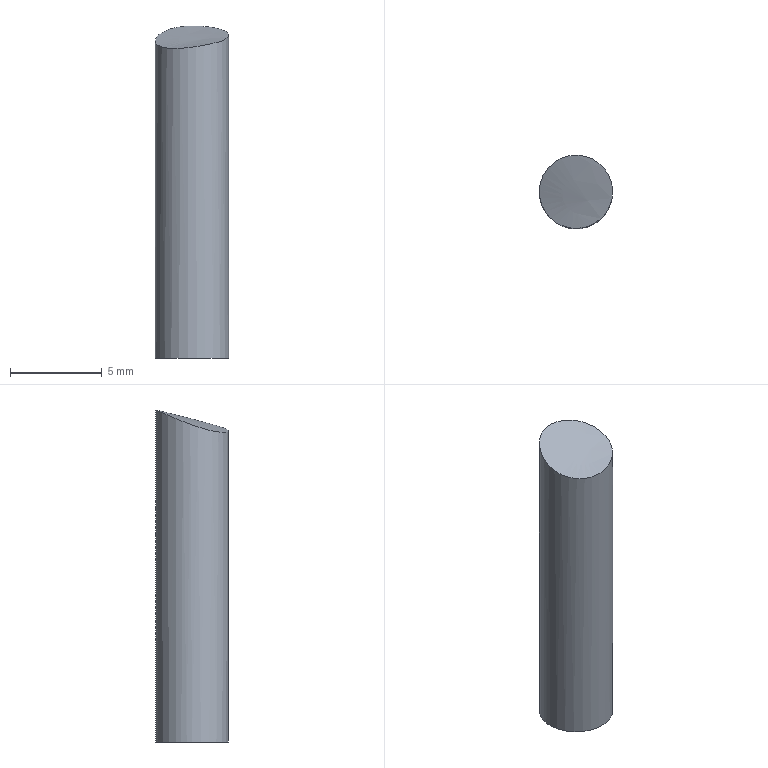Part | NX | features solid 2 | 1 solid | 3 faces | box 4.003 x 4 x 18.114 mm | volume 219.857 mm3 | plane 1 | spline 1 | cylinder 1 | commonest cylinder face diameters 4 x1
STEP:
#1=CARTESIAN_POINT('',(682.588,-10.702,-23.));
#2=VERTEX_POINT('',#1);
#3=CARTESIAN_POINT('',(684.588,-10.702,-23.));
#4=DIRECTION('',(0.,0.,1.));
#5=DIRECTION('',(-1.,0.,0.));
#6=AXIS2_PLACEMENT_3D('',#3,#4,#5);
#7=CIRCLE('',#6,2.);
#8=EDGE_CURVE('',#2,#2,#7,.T.);
#9=ORIENTED_EDGE('',*,*,#8,.F.);
#10=EDGE_LOOP('',(#9));
#11=FACE_BOUND('',#10,.T.);
#12=CARTESIAN_POINT('',(684.588,-10.702,-23.));
#13=DIRECTION('',(0.,0.,-1.));
#14=DIRECTION('',(1.,0.,0.));
#15=AXIS2_PLACEMENT_3D('',#12,#13,#14);
#16=PLANE('',#15);
#17=ADVANCED_FACE('',(#11),#16,.T.);
#18=CARTESIAN_POINT('',(682.787,-9.833,-5.361));
#19=VERTEX_POINT('',#18);
#20=CARTESIAN_POINT('',(682.477,-11.353,-5.969));
#21=CARTESIAN_POINT('',(682.608,-9.756,-5.337));
#22=CARTESIAN_POINT('',(683.815,-8.618,-4.849));
#23=CARTESIAN_POINT('',(685.572,-8.702,-4.891));
#24=CARTESIAN_POINT('',(686.688,-10.003,-5.195));
#25=CARTESIAN_POINT('',(686.578,-11.667,-5.637));
#26=CARTESIAN_POINT('',(685.317,-12.801,-5.954));
#27=CARTESIAN_POINT('',(683.582,-12.693,-6.19));
#28=CARTESIAN_POINT('',(682.477,-11.353,-5.969));
#29=CARTESIAN_POINT('',(682.608,-9.756,-5.337));
#30=CARTESIAN_POINT('',(683.815,-8.618,-4.849));
#31=B_SPLINE_CURVE_WITH_KNOTS('',3,(#20,#21,#22,#23,#24,#25,#26,#27,#28,#29,#30),.UNSPECIFIED.,.T.,.F.,(1,1,1,1,1,1,1,1,1,1,1,1,1,1,1),(-0.004799,-0.0032,-0.0016,0.,0.0016,0.0032,0.004799,0.006399,0.007999,0.009599,0.0112,0.0128,0.0144,0.016,0.0176),.UNSPECIFIED.);
#32=EDGE_CURVE('',#19,#19,#31,.T.);
#33=ORIENTED_EDGE('',*,*,#32,.F.);
#34=EDGE_LOOP('',(#33));
#35=FACE_BOUND('',#34,.T.);
#36=CARTESIAN_POINT('',(671.633,-2.461,-7.124));
#37=CARTESIAN_POINT('',(672.268,-2.468,-7.039));
#38=CARTESIAN_POINT('',(672.897,-2.479,-6.903));
#39=CARTESIAN_POINT('',(673.513,-2.494,-6.717));
#40=CARTESIAN_POINT('',(674.112,-2.513,-6.483));
#41=CARTESIAN_POINT('',(674.688,-2.535,-6.203));
#42=CARTESIAN_POINT('',(675.365,-2.562,-5.873));
#43=CARTESIAN_POINT('',(676.043,-2.588,-5.544));
#44=CARTESIAN_POINT('',(676.72,-2.615,-5.214));
#45=CARTESIAN_POINT('',(677.398,-2.641,-4.885));
#46=CARTESIAN_POINT('',(678.075,-2.668,-4.555));
#47=CARTESIAN_POINT('',(671.632,-4.157,-7.26));
#48=CARTESIAN_POINT('',(672.267,-4.072,-7.167));
#49=CARTESIAN_POINT('',(672.895,-3.991,-7.024));
#50=CARTESIAN_POINT('',(673.511,-3.915,-6.832));
#51=CARTESIAN_POINT('',(674.11,-3.845,-6.59));
#52=CARTESIAN_POINT('',(674.686,-3.78,-6.304));
#53=CARTESIAN_POINT('',(675.363,-3.704,-5.966));
#54=CARTESIAN_POINT('',(676.04,-3.629,-5.629));
#55=CARTESIAN_POINT('',(676.718,-3.553,-5.291));
#56=CARTESIAN_POINT('',(677.395,-3.477,-4.954));
#57=CARTESIAN_POINT('',(678.072,-3.401,-4.616));
#58=CARTESIAN_POINT('',(671.939,-5.86,-7.355));
#59=CARTESIAN_POINT('',(672.555,-5.682,-7.257));
#60=CARTESIAN_POINT('',(673.163,-5.508,-7.11));
#61=CARTESIAN_POINT('',(673.76,-5.34,-6.913));
#62=CARTESIAN_POINT('',(674.34,-5.179,-6.668));
#63=CARTESIAN_POINT('',(674.898,-5.026,-6.379));
#64=CARTESIAN_POINT('',(675.554,-4.846,-6.038));
#65=CARTESIAN_POINT('',(676.21,-4.667,-5.697));
#66=CARTESIAN_POINT('',(676.866,-4.487,-5.356));
#67=CARTESIAN_POINT('',(677.522,-4.307,-5.015));
#68=CARTESIAN_POINT('',(678.178,-4.127,-4.674));
#69=CARTESIAN_POINT('',(672.552,-7.478,-7.402));
#70=CARTESIAN_POINT('',(673.129,-7.214,-7.303));
#71=CARTESIAN_POINT('',(673.699,-6.955,-7.154));
#72=CARTESIAN_POINT('',(674.258,-6.701,-6.957));
#73=CARTESIAN_POINT('',(674.801,-6.456,-6.713));
#74=CARTESIAN_POINT('',(675.323,-6.222,-6.424));
#75=CARTESIAN_POINT('',(675.937,-5.945,-6.085));
#76=CARTESIAN_POINT('',(676.551,-5.669,-5.746));
#77=CARTESIAN_POINT('',(677.165,-5.393,-5.407));
#78=CARTESIAN_POINT('',(677.779,-5.117,-5.068));
#79=CARTESIAN_POINT('',(678.393,-4.841,-4.728));
#80=CARTESIAN_POINT('',(674.103,-10.038,-7.396));
#81=CARTESIAN_POINT('',(674.583,-9.642,-7.298));
#82=CARTESIAN_POINT('',(675.057,-9.251,-7.153));
#83=CARTESIAN_POINT('',(675.521,-8.866,-6.962));
#84=CARTESIAN_POINT('',(675.97,-8.491,-6.726));
#85=CARTESIAN_POINT('',(676.403,-8.129,-6.448));
#86=CARTESIAN_POINT('',(676.911,-7.703,-6.121));
#87=CARTESIAN_POINT('',(677.42,-7.277,-5.793));
#88=CARTESIAN_POINT('',(677.928,-6.851,-5.466));
#89=CARTESIAN_POINT('',(678.437,-6.426,-5.139));
#90=CARTESIAN_POINT('',(678.945,-6.,-4.811));
#91=CARTESIAN_POINT('',(676.32,-11.949,-7.241));
#92=CARTESIAN_POINT('',(676.667,-11.467,-7.153));
#93=CARTESIAN_POINT('',(677.008,-10.988,-7.022));
#94=CARTESIAN_POINT('',(677.34,-10.516,-6.848));
#95=CARTESIAN_POINT('',(677.661,-10.054,-6.632));
#96=CARTESIAN_POINT('',(677.969,-9.607,-6.376));
#97=CARTESIAN_POINT('',(678.331,-9.081,-6.075));
#98=CARTESIAN_POINT('',(678.693,-8.555,-5.774));
#99=CARTESIAN_POINT('',(679.055,-8.029,-5.473));
#100=CARTESIAN_POINT('',(679.417,-7.502,-5.172));
#101=CARTESIAN_POINT('',(679.779,-6.976,-4.871));
#102=CARTESIAN_POINT('',(677.364,-12.624,-7.148));
#103=CARTESIAN_POINT('',(677.65,-12.114,-7.067));
#104=CARTESIAN_POINT('',(677.929,-11.607,-6.943));
#105=CARTESIAN_POINT('',(678.201,-11.107,-6.778));
#106=CARTESIAN_POINT('',(678.462,-10.618,-6.572));
#107=CARTESIAN_POINT('',(678.712,-10.143,-6.328));
#108=CARTESIAN_POINT('',(679.006,-9.584,-6.041));
#109=CARTESIAN_POINT('',(679.3,-9.026,-5.754));
#110=CARTESIAN_POINT('',(679.594,-8.467,-5.466));
#111=CARTESIAN_POINT('',(679.888,-7.908,-5.179));
#112=CARTESIAN_POINT('',(680.182,-7.35,-4.892));
#113=CARTESIAN_POINT('',(679.743,-13.727,-6.898));
#114=CARTESIAN_POINT('',(679.892,-13.181,-6.832));
#115=CARTESIAN_POINT('',(680.035,-12.638,-6.728));
#116=CARTESIAN_POINT('',(680.171,-12.101,-6.586));
#117=CARTESIAN_POINT('',(680.3,-11.575,-6.406));
#118=CARTESIAN_POINT('',(680.421,-11.062,-6.191));
#119=CARTESIAN_POINT('',(680.563,-10.459,-5.938));
#120=CARTESIAN_POINT('',(680.706,-9.856,-5.684));
#121=CARTESIAN_POINT('',(680.848,-9.252,-5.431));
#122=CARTESIAN_POINT('',(680.99,-8.649,-5.178));
#123=CARTESIAN_POINT('',(681.132,-8.046,-4.925));
#124=CARTESIAN_POINT('',(682.276,-14.076,-6.555));
#125=CARTESIAN_POINT('',(682.288,-13.541,-6.51));
#126=CARTESIAN_POINT('',(682.296,-13.01,-6.431));
#127=CARTESIAN_POINT('',(682.298,-12.484,-6.317));
#128=CARTESIAN_POINT('',(682.296,-11.967,-6.169));
#129=CARTESIAN_POINT('',(682.288,-11.462,-5.989));
#130=CARTESIAN_POINT('',(682.279,-10.868,-5.778));
#131=CARTESIAN_POINT('',(682.27,-10.274,-5.566));
#132=CARTESIAN_POINT('',(682.26,-9.68,-5.354));
#133=CARTESIAN_POINT('',(682.251,-9.086,-5.143));
#134=CARTESIAN_POINT('',(682.242,-8.492,-4.931));
#135=CARTESIAN_POINT('',(683.618,-14.039,-6.353));
#136=CARTESIAN_POINT('',(683.562,-13.524,-6.319));
#137=CARTESIAN_POINT('',(683.502,-13.012,-6.254));
#138=CARTESIAN_POINT('',(683.437,-12.505,-6.156));
#139=CARTESIAN_POINT('',(683.368,-12.006,-6.027));
#140=CARTESIAN_POINT('',(683.295,-11.518,-5.867));
#141=CARTESIAN_POINT('',(683.21,-10.945,-5.679));
#142=CARTESIAN_POINT('',(683.124,-10.371,-5.491));
#143=CARTESIAN_POINT('',(683.039,-9.797,-5.303));
#144=CARTESIAN_POINT('',(682.953,-9.224,-5.115));
#145=CARTESIAN_POINT('',(682.868,-8.65,-4.926));
#146=CARTESIAN_POINT('',(686.716,-13.436,-5.837));
#147=CARTESIAN_POINT('',(686.515,-12.997,-5.832));
#148=CARTESIAN_POINT('',(686.31,-12.561,-5.8));
#149=CARTESIAN_POINT('',(686.103,-12.128,-5.742));
#150=CARTESIAN_POINT('',(685.893,-11.701,-5.657));
#151=CARTESIAN_POINT('',(685.682,-11.283,-5.547));
#152=CARTESIAN_POINT('',(685.434,-10.79,-5.416));
#153=CARTESIAN_POINT('',(685.186,-10.298,-5.286));
#154=CARTESIAN_POINT('',(684.938,-9.805,-5.156));
#155=CARTESIAN_POINT('',(684.689,-9.313,-5.025));
#156=CARTESIAN_POINT('',(684.441,-8.82,-4.895));
#157=CARTESIAN_POINT('',(689.23,-11.783,-5.313));
#158=CARTESIAN_POINT('',(688.945,-11.467,-5.332));
#159=CARTESIAN_POINT('',(688.657,-11.152,-5.329));
#160=CARTESIAN_POINT('',(688.367,-10.84,-5.306));
#161=CARTESIAN_POINT('',(688.076,-10.531,-5.262));
#162=CARTESIAN_POINT('',(687.784,-10.228,-5.197));
#163=CARTESIAN_POINT('',(687.441,-9.871,-5.121));
#164=CARTESIAN_POINT('',(687.099,-9.514,-5.044));
#165=CARTESIAN_POINT('',(686.756,-9.157,-4.968));
#166=CARTESIAN_POINT('',(686.413,-8.801,-4.891));
#167=CARTESIAN_POINT('',(686.07,-8.444,-4.815));
#168=CARTESIAN_POINT('',(690.384,-10.54,-5.03));
#169=CARTESIAN_POINT('',(690.078,-10.301,-5.059));
#170=CARTESIAN_POINT('',(689.769,-10.064,-5.07));
#171=CARTESIAN_POINT('',(689.458,-9.829,-5.064));
#172=CARTESIAN_POINT('',(689.146,-9.597,-5.039));
#173=CARTESIAN_POINT('',(688.834,-9.368,-4.997));
#174=CARTESIAN_POINT('',(688.467,-9.098,-4.948));
#175=CARTESIAN_POINT('',(688.101,-8.829,-4.899));
#176=CARTESIAN_POINT('',(687.734,-8.56,-4.849));
#177=CARTESIAN_POINT('',(687.367,-8.29,-4.8));
#178=CARTESIAN_POINT('',(687.001,-8.021,-4.75));
#179=CARTESIAN_POINT('',(691.807,-8.172,-4.612));
#180=CARTESIAN_POINT('',(691.505,-8.051,-4.651));
#181=CARTESIAN_POINT('',(691.201,-7.931,-4.677));
#182=CARTESIAN_POINT('',(690.895,-7.813,-4.69));
#183=CARTESIAN_POINT('',(690.589,-7.695,-4.691));
#184=CARTESIAN_POINT('',(690.283,-7.58,-4.679));
#185=CARTESIAN_POINT('',(689.923,-7.444,-4.665));
#186=CARTESIAN_POINT('',(689.563,-7.308,-4.651));
#187=CARTESIAN_POINT('',(689.203,-7.172,-4.637));
#188=CARTESIAN_POINT('',(688.843,-7.036,-4.623));
#189=CARTESIAN_POINT('',(688.483,-6.9,-4.609));
#190=CARTESIAN_POINT('',(692.404,-5.77,-4.322));
#191=CARTESIAN_POINT('',(692.137,-5.72,-4.361));
#192=CARTESIAN_POINT('',(691.869,-5.67,-4.391));
#193=CARTESIAN_POINT('',(691.6,-5.621,-4.411));
#194=CARTESIAN_POINT('',(691.33,-5.573,-4.423));
#195=CARTESIAN_POINT('',(691.06,-5.526,-4.425));
#196=CARTESIAN_POINT('',(690.743,-5.471,-4.428));
#197=CARTESIAN_POINT('',(690.425,-5.416,-4.43));
#198=CARTESIAN_POINT('',(690.107,-5.36,-4.433));
#199=CARTESIAN_POINT('',(689.79,-5.305,-4.436));
#200=CARTESIAN_POINT('',(689.472,-5.25,-4.438));
#201=CARTESIAN_POINT('',(692.538,-4.76,-4.219));
#202=CARTESIAN_POINT('',(692.287,-4.729,-4.257));
#203=CARTESIAN_POINT('',(692.035,-4.699,-4.287));
#204=CARTESIAN_POINT('',(691.781,-4.669,-4.309));
#205=CARTESIAN_POINT('',(691.527,-4.641,-4.322));
#206=CARTESIAN_POINT('',(691.273,-4.612,-4.328));
#207=CARTESIAN_POINT('',(690.974,-4.579,-4.335));
#208=CARTESIAN_POINT('',(690.675,-4.546,-4.341));
#209=CARTESIAN_POINT('',(690.376,-4.513,-4.348));
#210=CARTESIAN_POINT('',(690.077,-4.48,-4.354));
#211=CARTESIAN_POINT('',(689.778,-4.447,-4.361));
#212=CARTESIAN_POINT('',(692.612,-3.786,-4.128));
#213=CARTESIAN_POINT('',(692.368,-3.767,-4.166));
#214=CARTESIAN_POINT('',(692.123,-3.749,-4.196));
#215=CARTESIAN_POINT('',(691.877,-3.732,-4.219));
#216=CARTESIAN_POINT('',(691.631,-3.716,-4.234));
#217=CARTESIAN_POINT('',(691.384,-3.7,-4.242));
#218=CARTESIAN_POINT('',(691.094,-3.681,-4.251));
#219=CARTESIAN_POINT('',(690.804,-3.663,-4.26));
#220=CARTESIAN_POINT('',(690.513,-3.644,-4.268));
#221=CARTESIAN_POINT('',(690.223,-3.625,-4.277));
#222=CARTESIAN_POINT('',(689.933,-3.607,-4.286));
#223=CARTESIAN_POINT('',(692.623,-2.801,-4.047));
#224=CARTESIAN_POINT('',(692.379,-2.795,-4.086));
#225=CARTESIAN_POINT('',(692.133,-2.79,-4.117));
#226=CARTESIAN_POINT('',(691.886,-2.785,-4.141));
#227=CARTESIAN_POINT('',(691.639,-2.781,-4.157));
#228=CARTESIAN_POINT('',(691.391,-2.778,-4.166));
#229=CARTESIAN_POINT('',(691.1,-2.774,-4.176));
#230=CARTESIAN_POINT('',(690.809,-2.77,-4.186));
#231=CARTESIAN_POINT('',(690.518,-2.766,-4.196));
#232=CARTESIAN_POINT('',(690.227,-2.762,-4.206));
#233=CARTESIAN_POINT('',(689.936,-2.758,-4.216));
#234=B_SPLINE_SURFACE_WITH_KNOTS('',5,5,((#36,#37,#38,#39,#40,#41,#42,#43,#44,#45,#46),(#47,#48,#49,#50,#51,#52,#53,#54,#55,#56,#57),(#58,#59,#60,#61,#62,#63,#64,#65,#66,#67,#68),(#69,#70,#71,#72,#73,#74,#75,#76,#77,#78,#79),(#80,#81,#82,#83,#84,#85,#86,#87,#88,#89,#90),(#91,#92,#93,#94,#95,#96,#97,#98,#99,#100,#101),(#102,#103,#104,#105,#106,#107,#108,#109,#110,#111,#112),(#113,#114,#115,#116,#117,#118,#119,#120,#121,#122,#123),(#124,#125,#126,#127,#128,#129,#130,#131,#132,#133,#134),(#135,#136,#137,#138,#139,#140,#141,#142,#143,#144,#145),(#146,#147,#148,#149,#150,#151,#152,#153,#154,#155,#156),(#157,#158,#159,#160,#161,#162,#163,#164,#165,#166,#167),(#168,#169,#170,#171,#172,#173,#174,#175,#176,#177,#178),(#179,#180,#181,#182,#183,#184,#185,#186,#187,#188,#189),(#190,#191,#192,#193,#194,#195,#196,#197,#198,#199,#200),(#201,#202,#203,#204,#205,#206,#207,#208,#209,#210,#211),(#212,#213,#214,#215,#216,#217,#218,#219,#220,#221,#222),(#223,#224,#225,#226,#227,#228,#229,#230,#231,#232,#233)),.UNSPECIFIED.,.F.,.F.,.F.,(6,3,3,3,3,6),(6,5,6),(0.,0.212,0.37,0.5499,0.8052,1.),(0.,1.,2.176),.UNSPECIFIED.);
#235=ADVANCED_FACE('',(#35),#234,.T.);
#236=ORIENTED_EDGE('',*,*,#8,.T.);
#237=EDGE_LOOP('',(#236));
#238=FACE_BOUND('',#237,.T.);
#239=ORIENTED_EDGE('',*,*,#32,.T.);
#240=EDGE_LOOP('',(#239));
#241=FACE_BOUND('',#240,.T.);
#242=CARTESIAN_POINT('',(684.588,-10.702,-3.));
#243=DIRECTION('',(0.,0.,-1.));
#244=DIRECTION('',(1.,0.,0.));
#245=AXIS2_PLACEMENT_3D('',#242,#243,#244);
#246=CYLINDRICAL_SURFACE('',#245,2.);
#247=ADVANCED_FACE('',(#238,#241),#246,.T.);
#248=CLOSED_SHELL('',(#17,#235,#247));
#249=MANIFOLD_SOLID_BREP('',#248);
#250=(LENGTH_UNIT()NAMED_UNIT(*)SI_UNIT(.MILLI.,.METRE.));
#251=UNCERTAINTY_MEASURE_WITH_UNIT(LENGTH_MEASURE(0.0508),#250,'','');
#252=(NAMED_UNIT(*)PLANE_ANGLE_UNIT()SI_UNIT($,.RADIAN.));
#253=(NAMED_UNIT(*)SI_UNIT($,.STERADIAN.)SOLID_ANGLE_UNIT());
#254=(GEOMETRIC_REPRESENTATION_CONTEXT(3)GLOBAL_UNCERTAINTY_ASSIGNED_CONTEXT((#251))GLOBAL_UNIT_ASSIGNED_CONTEXT((#250,#252,#253))REPRESENTATION_CONTEXT('',''));
#255=ADVANCED_BREP_SHAPE_REPRESENTATION('',(#249),#254);